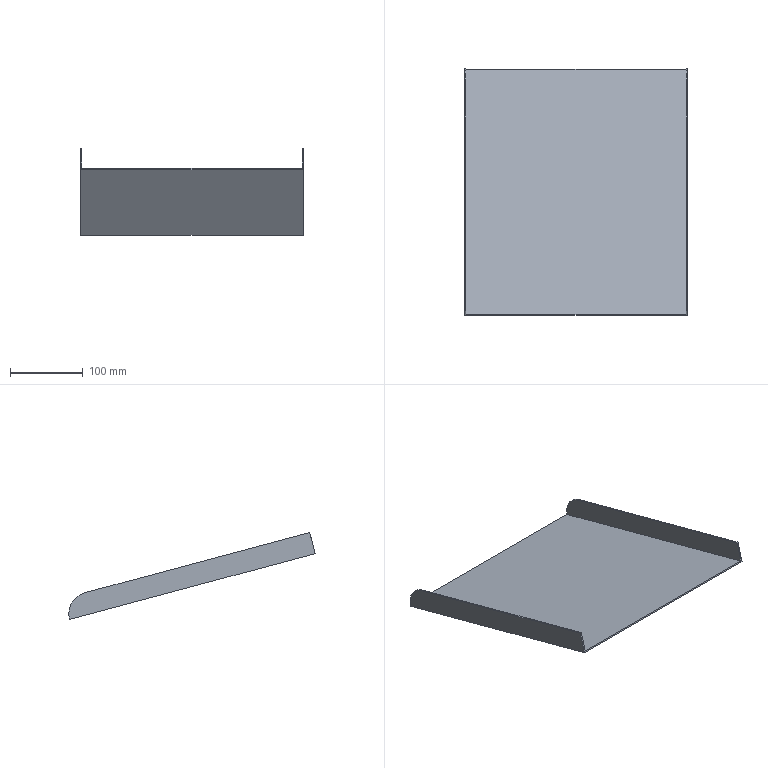Part | NX | features solid 2 | 1 solid | 12 faces | box 306.72 x 339.096 x 119.564 mm | volume 253131 mm3 | plane 10 | cylinder 2 | commonest cylinder face diameters 60 x2
STEP:
#1=CARTESIAN_POINT('',(88.964,801.67,-479.689));
#2=VERTEX_POINT('',#1);
#3=CARTESIAN_POINT('',(88.964,1139.679,-570.258));
#4=VERTEX_POINT('',#3);
#5=CARTESIAN_POINT('',(88.964,975.536,-526.276));
#6=DIRECTION('',(0.,0.9659,-0.2588));
#7=VECTOR('',#6,1000.);
#8=LINE('',#5,#7);
#9=EDGE_CURVE('',#2,#4,#8,.T.);
#10=ORIENTED_EDGE('',*,*,#9,.F.);
#11=CARTESIAN_POINT('',(391.683,801.67,-479.689));
#12=VERTEX_POINT('',#11);
#13=CARTESIAN_POINT('',(98.964,801.67,-479.689));
#14=DIRECTION('',(-1.,0.,0.));
#15=VECTOR('',#14,1000.);
#16=LINE('',#13,#15);
#17=EDGE_CURVE('',#2,#12,#16,.F.);
#18=ORIENTED_EDGE('',*,*,#17,.T.);
#19=CARTESIAN_POINT('',(391.683,1139.679,-570.258));
#20=VERTEX_POINT('',#19);
#21=CARTESIAN_POINT('',(391.683,975.536,-526.276));
#22=DIRECTION('',(0.,0.9659,-0.2588));
#23=VECTOR('',#22,1000.);
#24=LINE('',#21,#23);
#25=EDGE_CURVE('',#12,#20,#24,.T.);
#26=ORIENTED_EDGE('',*,*,#25,.T.);
#27=CARTESIAN_POINT('',(393.683,1139.679,-570.258));
#28=VERTEX_POINT('',#27);
#29=CARTESIAN_POINT('',(403.683,1139.679,-570.258));
#30=DIRECTION('',(1.,0.,0.));
#31=VECTOR('',#30,1000.);
#32=LINE('',#29,#31);
#33=EDGE_CURVE('',#28,#20,#32,.F.);
#34=ORIENTED_EDGE('',*,*,#33,.F.);
#35=CARTESIAN_POINT('',(393.683,1139.744,-570.276));
#36=VERTEX_POINT('',#35);
#37=CARTESIAN_POINT('',(393.683,975.536,-526.276));
#38=DIRECTION('',(0.,-0.9659,0.2588));
#39=VECTOR('',#38,1000.);
#40=LINE('',#37,#39);
#41=EDGE_CURVE('',#28,#36,#40,.F.);
#42=ORIENTED_EDGE('',*,*,#41,.T.);
#43=CARTESIAN_POINT('',(86.964,1139.744,-570.276));
#44=VERTEX_POINT('',#43);
#45=CARTESIAN_POINT('',(98.964,1139.744,-570.276));
#46=DIRECTION('',(1.,0.,0.));
#47=VECTOR('',#46,1000.);
#48=LINE('',#45,#47);
#49=EDGE_CURVE('',#44,#36,#48,.T.);
#50=ORIENTED_EDGE('',*,*,#49,.F.);
#51=CARTESIAN_POINT('',(86.964,1139.679,-570.258));
#52=VERTEX_POINT('',#51);
#53=CARTESIAN_POINT('',(86.964,975.536,-526.276));
#54=DIRECTION('',(0.,0.9659,-0.2588));
#55=VECTOR('',#54,1000.);
#56=LINE('',#53,#55);
#57=EDGE_CURVE('',#52,#44,#56,.T.);
#58=ORIENTED_EDGE('',*,*,#57,.F.);
#59=CARTESIAN_POINT('',(86.964,1139.679,-570.258));
#60=DIRECTION('',(-1.,0.,0.));
#61=VECTOR('',#60,1000.);
#62=LINE('',#59,#61);
#63=EDGE_CURVE('',#4,#52,#62,.T.);
#64=ORIENTED_EDGE('',*,*,#63,.F.);
#65=EDGE_LOOP('',(#10,#18,#26,#34,#42,#50,#58,#64));
#66=FACE_BOUND('',#65,.T.);
#67=CARTESIAN_POINT('',(98.964,975.536,-526.276));
#68=DIRECTION('',(0.,0.2588,0.9659));
#69=DIRECTION('',(1.,0.,0.));
#70=AXIS2_PLACEMENT_3D('',#67,#68,#69);
#71=PLANE('',#70);
#72=ADVANCED_FACE('',(#66),#71,.T.);
#73=ORIENTED_EDGE('',*,*,#17,.F.);
#74=CARTESIAN_POINT('',(88.964,808.917,-452.643));
#75=VERTEX_POINT('',#74);
#76=CARTESIAN_POINT('',(88.964,801.152,-481.621));
#77=DIRECTION('',(0.,-0.2588,-0.9659));
#78=VECTOR('',#77,1000.);
#79=LINE('',#76,#78);
#80=EDGE_CURVE('',#2,#75,#79,.F.);
#81=ORIENTED_EDGE('',*,*,#80,.T.);
#82=CARTESIAN_POINT('',(86.964,808.917,-452.643));
#83=VERTEX_POINT('',#82);
#84=CARTESIAN_POINT('',(98.964,808.917,-452.643));
#85=DIRECTION('',(1.,0.,0.));
#86=VECTOR('',#85,1000.);
#87=LINE('',#84,#86);
#88=EDGE_CURVE('',#83,#75,#87,.T.);
#89=ORIENTED_EDGE('',*,*,#88,.F.);
#90=CARTESIAN_POINT('',(86.964,801.152,-481.621));
#91=VERTEX_POINT('',#90);
#92=CARTESIAN_POINT('',(86.964,801.67,-479.689));
#93=DIRECTION('',(0.,0.2588,0.9659));
#94=VECTOR('',#93,1000.);
#95=LINE('',#92,#94);
#96=EDGE_CURVE('',#83,#91,#95,.F.);
#97=ORIENTED_EDGE('',*,*,#96,.T.);
#98=CARTESIAN_POINT('',(393.683,801.152,-481.621));
#99=VERTEX_POINT('',#98);
#100=CARTESIAN_POINT('',(98.964,801.152,-481.621));
#101=DIRECTION('',(-1.,0.,0.));
#102=VECTOR('',#101,1000.);
#103=LINE('',#100,#102);
#104=EDGE_CURVE('',#91,#99,#103,.F.);
#105=ORIENTED_EDGE('',*,*,#104,.T.);
#106=CARTESIAN_POINT('',(393.683,808.917,-452.643));
#107=VERTEX_POINT('',#106);
#108=CARTESIAN_POINT('',(393.683,801.67,-479.689));
#109=DIRECTION('',(0.,-0.2588,-0.9659));
#110=VECTOR('',#109,1000.);
#111=LINE('',#108,#110);
#112=EDGE_CURVE('',#107,#99,#111,.T.);
#113=ORIENTED_EDGE('',*,*,#112,.F.);
#114=CARTESIAN_POINT('',(391.683,808.917,-452.643));
#115=VERTEX_POINT('',#114);
#116=CARTESIAN_POINT('',(98.964,808.917,-452.643));
#117=DIRECTION('',(1.,0.,0.));
#118=VECTOR('',#117,1000.);
#119=LINE('',#116,#118);
#120=EDGE_CURVE('',#107,#115,#119,.F.);
#121=ORIENTED_EDGE('',*,*,#120,.T.);
#122=CARTESIAN_POINT('',(391.683,801.152,-481.621));
#123=DIRECTION('',(0.,-0.2588,-0.9659));
#124=VECTOR('',#123,1000.);
#125=LINE('',#122,#124);
#126=EDGE_CURVE('',#12,#115,#125,.F.);
#127=ORIENTED_EDGE('',*,*,#126,.F.);
#128=EDGE_LOOP('',(#73,#81,#89,#97,#105,#113,#121,#127));
#129=FACE_BOUND('',#128,.T.);
#130=CARTESIAN_POINT('',(98.964,801.67,-479.689));
#131=DIRECTION('',(0.,-0.9659,0.2588));
#132=DIRECTION('',(1.,0.,0.));
#133=AXIS2_PLACEMENT_3D('',#130,#131,#132);
#134=PLANE('',#133);
#135=ADVANCED_FACE('',(#129),#134,.T.);
#136=ORIENTED_EDGE('',*,*,#41,.F.);
#137=CARTESIAN_POINT('',(393.683,1118.013,-535.465));
#138=VERTEX_POINT('',#137);
#139=CARTESIAN_POINT('',(393.683,1110.248,-564.443));
#140=DIRECTION('',(1.,0.,0.));
#141=DIRECTION('',(0.,0.,-1.));
#142=AXIS2_PLACEMENT_3D('',#139,#140,#141);
#143=CIRCLE('',#142,30.);
#144=EDGE_CURVE('',#28,#138,#143,.T.);
#145=ORIENTED_EDGE('',*,*,#144,.T.);
#146=CARTESIAN_POINT('',(393.683,953.805,-491.466));
#147=DIRECTION('',(0.,-0.9659,0.2588));
#148=VECTOR('',#147,1000.);
#149=LINE('',#146,#148);
#150=EDGE_CURVE('',#107,#138,#149,.F.);
#151=ORIENTED_EDGE('',*,*,#150,.F.);
#152=ORIENTED_EDGE('',*,*,#112,.T.);
#153=CARTESIAN_POINT('',(393.683,1139.226,-572.207));
#154=VERTEX_POINT('',#153);
#155=CARTESIAN_POINT('',(393.683,975.019,-528.208));
#156=DIRECTION('',(0.,-0.9659,0.2588));
#157=VECTOR('',#156,1000.);
#158=LINE('',#155,#157);
#159=EDGE_CURVE('',#99,#154,#158,.F.);
#160=ORIENTED_EDGE('',*,*,#159,.T.);
#161=CARTESIAN_POINT('',(393.683,1139.744,-570.276));
#162=DIRECTION('',(0.,0.2588,0.9659));
#163=VECTOR('',#162,1000.);
#164=LINE('',#161,#163);
#165=EDGE_CURVE('',#36,#154,#164,.F.);
#166=ORIENTED_EDGE('',*,*,#165,.F.);
#167=EDGE_LOOP('',(#136,#145,#151,#152,#160,#166));
#168=FACE_BOUND('',#167,.T.);
#169=CARTESIAN_POINT('',(393.683,975.536,-526.276));
#170=DIRECTION('',(1.,0.,0.));
#171=DIRECTION('',(0.,0.9659,-0.2588));
#172=AXIS2_PLACEMENT_3D('',#169,#170,#171);
#173=PLANE('',#172);
#174=ADVANCED_FACE('',(#168),#173,.T.);
#175=ORIENTED_EDGE('',*,*,#165,.T.);
#176=CARTESIAN_POINT('',(86.964,1139.226,-572.207));
#177=VERTEX_POINT('',#176);
#178=CARTESIAN_POINT('',(98.964,1139.226,-572.207));
#179=DIRECTION('',(1.,0.,0.));
#180=VECTOR('',#179,1000.);
#181=LINE('',#178,#180);
#182=EDGE_CURVE('',#177,#154,#181,.T.);
#183=ORIENTED_EDGE('',*,*,#182,.F.);
#184=CARTESIAN_POINT('',(86.964,1139.744,-570.276));
#185=DIRECTION('',(0.,-0.2588,-0.9659));
#186=VECTOR('',#185,1000.);
#187=LINE('',#184,#186);
#188=EDGE_CURVE('',#44,#177,#187,.T.);
#189=ORIENTED_EDGE('',*,*,#188,.F.);
#190=ORIENTED_EDGE('',*,*,#49,.T.);
#191=EDGE_LOOP('',(#175,#183,#189,#190));
#192=FACE_BOUND('',#191,.T.);
#193=CARTESIAN_POINT('',(98.964,1139.744,-570.276));
#194=DIRECTION('',(0.,-0.9659,0.2588));
#195=DIRECTION('',(1.,0.,0.));
#196=AXIS2_PLACEMENT_3D('',#193,#194,#195);
#197=PLANE('',#196);
#198=ADVANCED_FACE('',(#192),#197,.F.);
#199=ORIENTED_EDGE('',*,*,#188,.T.);
#200=CARTESIAN_POINT('',(86.964,975.019,-528.208));
#201=DIRECTION('',(0.,0.9659,-0.2588));
#202=VECTOR('',#201,1000.);
#203=LINE('',#200,#202);
#204=EDGE_CURVE('',#91,#177,#203,.T.);
#205=ORIENTED_EDGE('',*,*,#204,.F.);
#206=ORIENTED_EDGE('',*,*,#96,.F.);
#207=CARTESIAN_POINT('',(86.964,1118.013,-535.465));
#208=VERTEX_POINT('',#207);
#209=CARTESIAN_POINT('',(86.964,953.805,-491.466));
#210=DIRECTION('',(0.,0.9659,-0.2588));
#211=VECTOR('',#210,1000.);
#212=LINE('',#209,#211);
#213=EDGE_CURVE('',#83,#208,#212,.T.);
#214=ORIENTED_EDGE('',*,*,#213,.T.);
#215=CARTESIAN_POINT('',(86.964,1110.248,-564.443));
#216=DIRECTION('',(1.,0.,0.));
#217=DIRECTION('',(0.,-0.2588,-0.9659));
#218=AXIS2_PLACEMENT_3D('',#215,#216,#217);
#219=CIRCLE('',#218,30.);
#220=EDGE_CURVE('',#208,#52,#219,.F.);
#221=ORIENTED_EDGE('',*,*,#220,.T.);
#222=ORIENTED_EDGE('',*,*,#57,.T.);
#223=EDGE_LOOP('',(#199,#205,#206,#214,#221,#222));
#224=FACE_BOUND('',#223,.T.);
#225=CARTESIAN_POINT('',(86.964,975.536,-526.276));
#226=DIRECTION('',(1.,0.,0.));
#227=DIRECTION('',(0.,0.9659,-0.2588));
#228=AXIS2_PLACEMENT_3D('',#225,#226,#227);
#229=PLANE('',#228);
#230=ADVANCED_FACE('',(#224),#229,.F.);
#231=ORIENTED_EDGE('',*,*,#159,.F.);
#232=ORIENTED_EDGE('',*,*,#104,.F.);
#233=ORIENTED_EDGE('',*,*,#204,.T.);
#234=ORIENTED_EDGE('',*,*,#182,.T.);
#235=EDGE_LOOP('',(#231,#232,#233,#234));
#236=FACE_BOUND('',#235,.T.);
#237=CARTESIAN_POINT('',(98.964,975.019,-528.208));
#238=DIRECTION('',(0.,0.2588,0.9659));
#239=DIRECTION('',(1.,0.,0.));
#240=AXIS2_PLACEMENT_3D('',#237,#238,#239);
#241=PLANE('',#240);
#242=ADVANCED_FACE('',(#236),#241,.F.);
#243=ORIENTED_EDGE('',*,*,#150,.T.);
#244=CARTESIAN_POINT('',(391.683,1118.013,-535.465));
#245=VERTEX_POINT('',#244);
#246=CARTESIAN_POINT('',(403.683,1118.013,-535.465));
#247=DIRECTION('',(1.,0.,0.));
#248=VECTOR('',#247,1000.);
#249=LINE('',#246,#248);
#250=EDGE_CURVE('',#138,#245,#249,.F.);
#251=ORIENTED_EDGE('',*,*,#250,.T.);
#252=CARTESIAN_POINT('',(391.683,953.805,-491.466));
#253=DIRECTION('',(0.,0.9659,-0.2588));
#254=VECTOR('',#253,1000.);
#255=LINE('',#252,#254);
#256=EDGE_CURVE('',#115,#245,#255,.T.);
#257=ORIENTED_EDGE('',*,*,#256,.F.);
#258=ORIENTED_EDGE('',*,*,#120,.F.);
#259=EDGE_LOOP('',(#243,#251,#257,#258));
#260=FACE_BOUND('',#259,.T.);
#261=CARTESIAN_POINT('',(403.683,953.805,-491.466));
#262=DIRECTION('',(0.,-0.2588,-0.9659));
#263=DIRECTION('',(0.,0.9659,-0.2588));
#264=AXIS2_PLACEMENT_3D('',#261,#262,#263);
#265=PLANE('',#264);
#266=ADVANCED_FACE('',(#260),#265,.F.);
#267=ORIENTED_EDGE('',*,*,#25,.F.);
#268=ORIENTED_EDGE('',*,*,#126,.T.);
#269=ORIENTED_EDGE('',*,*,#256,.T.);
#270=CARTESIAN_POINT('',(391.683,1110.248,-564.443));
#271=DIRECTION('',(1.,0.,0.));
#272=DIRECTION('',(0.,0.,-1.));
#273=AXIS2_PLACEMENT_3D('',#270,#271,#272);
#274=CIRCLE('',#273,30.);
#275=EDGE_CURVE('',#245,#20,#274,.F.);
#276=ORIENTED_EDGE('',*,*,#275,.T.);
#277=EDGE_LOOP('',(#267,#268,#269,#276));
#278=FACE_BOUND('',#277,.T.);
#279=CARTESIAN_POINT('',(391.683,946.041,-520.444));
#280=DIRECTION('',(1.,0.,0.));
#281=DIRECTION('',(0.,-0.2588,-0.9659));
#282=AXIS2_PLACEMENT_3D('',#279,#280,#281);
#283=PLANE('',#282);
#284=ADVANCED_FACE('',(#278),#283,.F.);
#285=ORIENTED_EDGE('',*,*,#144,.F.);
#286=ORIENTED_EDGE('',*,*,#33,.T.);
#287=ORIENTED_EDGE('',*,*,#275,.F.);
#288=ORIENTED_EDGE('',*,*,#250,.F.);
#289=EDGE_LOOP('',(#285,#286,#287,#288));
#290=FACE_BOUND('',#289,.T.);
#291=CARTESIAN_POINT('',(403.683,1110.248,-564.443));
#292=DIRECTION('',(1.,0.,0.));
#293=DIRECTION('',(0.,-0.2588,-0.9659));
#294=AXIS2_PLACEMENT_3D('',#291,#292,#293);
#295=CYLINDRICAL_SURFACE('',#294,30.);
#296=ADVANCED_FACE('',(#290),#295,.T.);
#297=CARTESIAN_POINT('',(88.964,1118.013,-535.465));
#298=VERTEX_POINT('',#297);
#299=CARTESIAN_POINT('',(88.964,953.805,-491.466));
#300=DIRECTION('',(0.,0.9659,-0.2588));
#301=VECTOR('',#300,1000.);
#302=LINE('',#299,#301);
#303=EDGE_CURVE('',#75,#298,#302,.T.);
#304=ORIENTED_EDGE('',*,*,#303,.T.);
#305=CARTESIAN_POINT('',(86.964,1118.013,-535.465));
#306=DIRECTION('',(1.,0.,0.));
#307=VECTOR('',#306,1000.);
#308=LINE('',#305,#307);
#309=EDGE_CURVE('',#298,#208,#308,.F.);
#310=ORIENTED_EDGE('',*,*,#309,.T.);
#311=ORIENTED_EDGE('',*,*,#213,.F.);
#312=ORIENTED_EDGE('',*,*,#88,.T.);
#313=EDGE_LOOP('',(#304,#310,#311,#312));
#314=FACE_BOUND('',#313,.T.);
#315=CARTESIAN_POINT('',(86.964,953.805,-491.466));
#316=DIRECTION('',(0.,-0.2588,-0.9659));
#317=DIRECTION('',(0.,0.9659,-0.2588));
#318=AXIS2_PLACEMENT_3D('',#315,#316,#317);
#319=PLANE('',#318);
#320=ADVANCED_FACE('',(#314),#319,.F.);
#321=ORIENTED_EDGE('',*,*,#80,.F.);
#322=ORIENTED_EDGE('',*,*,#9,.T.);
#323=CARTESIAN_POINT('',(88.964,1110.248,-564.443));
#324=DIRECTION('',(1.,0.,0.));
#325=DIRECTION('',(0.,-0.2588,-0.9659));
#326=AXIS2_PLACEMENT_3D('',#323,#324,#325);
#327=CIRCLE('',#326,30.);
#328=EDGE_CURVE('',#4,#298,#327,.T.);
#329=ORIENTED_EDGE('',*,*,#328,.T.);
#330=ORIENTED_EDGE('',*,*,#303,.F.);
#331=EDGE_LOOP('',(#321,#322,#329,#330));
#332=FACE_BOUND('',#331,.T.);
#333=CARTESIAN_POINT('',(88.964,946.041,-520.444));
#334=DIRECTION('',(1.,0.,0.));
#335=DIRECTION('',(0.,-0.2588,-0.9659));
#336=AXIS2_PLACEMENT_3D('',#333,#334,#335);
#337=PLANE('',#336);
#338=ADVANCED_FACE('',(#332),#337,.T.);
#339=ORIENTED_EDGE('',*,*,#328,.F.);
#340=ORIENTED_EDGE('',*,*,#63,.T.);
#341=ORIENTED_EDGE('',*,*,#220,.F.);
#342=ORIENTED_EDGE('',*,*,#309,.F.);
#343=EDGE_LOOP('',(#339,#340,#341,#342));
#344=FACE_BOUND('',#343,.T.);
#345=CARTESIAN_POINT('',(86.964,1110.248,-564.443));
#346=DIRECTION('',(-1.,0.,0.));
#347=DIRECTION('',(0.,0.2588,0.9659));
#348=AXIS2_PLACEMENT_3D('',#345,#346,#347);
#349=CYLINDRICAL_SURFACE('',#348,30.);
#350=ADVANCED_FACE('',(#344),#349,.T.);
#351=CLOSED_SHELL('',(#72,#135,#174,#198,#230,#242,#266,#284,#296,#320,#338,#350));
#352=MANIFOLD_SOLID_BREP('',#351);
#353=(LENGTH_UNIT()NAMED_UNIT(*)SI_UNIT(.MILLI.,.METRE.));
#354=UNCERTAINTY_MEASURE_WITH_UNIT(LENGTH_MEASURE(0.00001),#353,'','');
#355=(NAMED_UNIT(*)PLANE_ANGLE_UNIT()SI_UNIT($,.RADIAN.));
#356=(NAMED_UNIT(*)SI_UNIT($,.STERADIAN.)SOLID_ANGLE_UNIT());
#357=(GEOMETRIC_REPRESENTATION_CONTEXT(3)GLOBAL_UNCERTAINTY_ASSIGNED_CONTEXT((#354))GLOBAL_UNIT_ASSIGNED_CONTEXT((#353,#355,#356))REPRESENTATION_CONTEXT('',''));
#358=ADVANCED_BREP_SHAPE_REPRESENTATION('',(#352),#357);